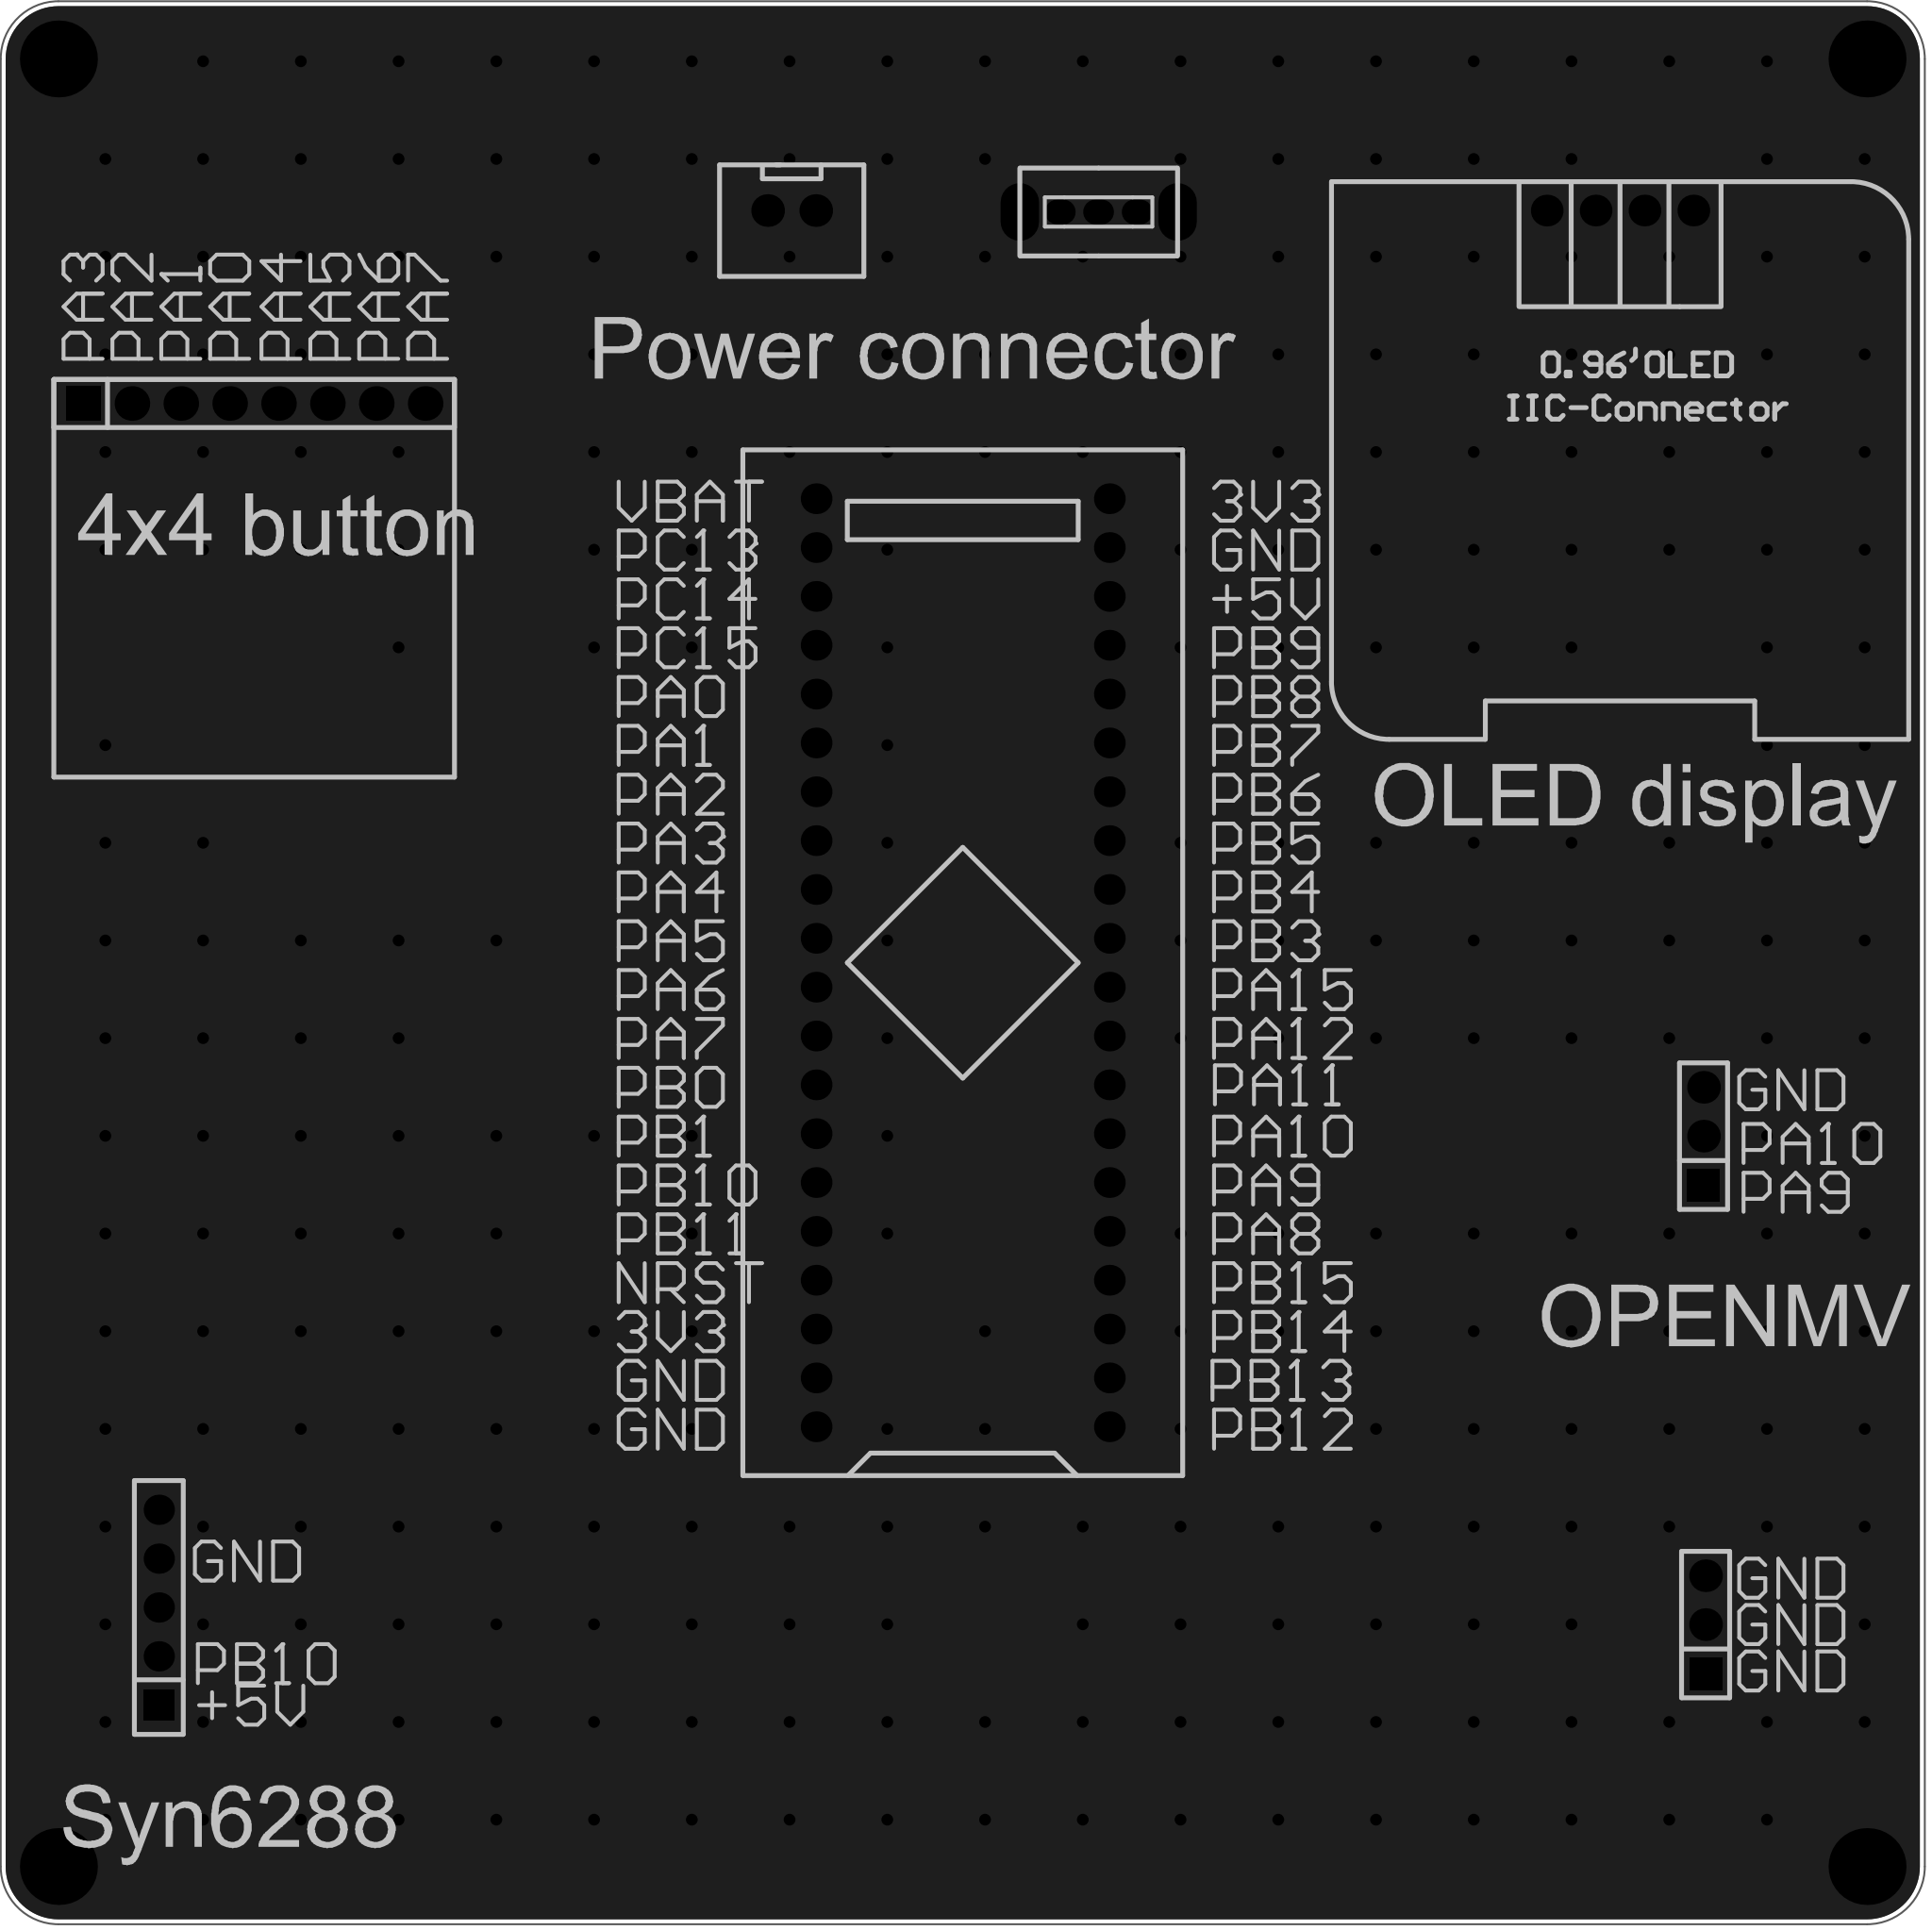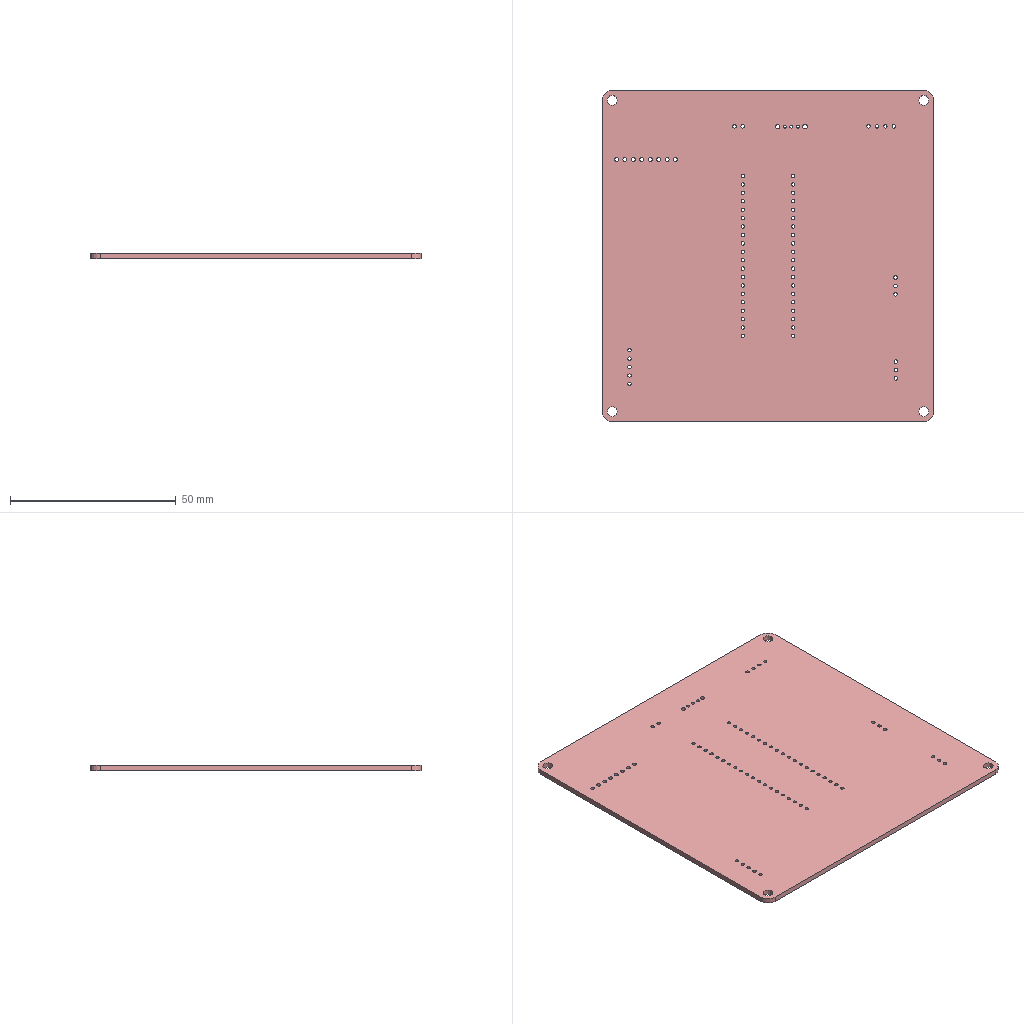Circuit board layout | Altium Designer | box 100 x 100 x 1.6 mm
Layer stack:
# Altium Designer layer stack of  (unit mm; dielectric type: 0 none, 1 core, 2 prepreg, 3 surface material)
index,name,kind,layer,copper_thickness_mm,dielectric_type,dielectric_thickness_mm,dielectric_material,dielectric_constant
0,Top Paste Mask Layer,other,,,,,,
1,Top Silkscreen Layer,other,,,,,,
2,Top Solder Mask Layer,dielectric,,,3,0.01,,3.3
3,Top Layer,copper,Top Layer,0.035,,,,
4,Dielectric1,dielectric,,,3,1.51,FR4,4.5
5,Bottom Layer,copper,Bottom Layer,0.035,,,,
6,Bottom Solder Mask Layer,dielectric,,,3,0.01,,3.3
7,Bottom Silkscreen Layer,other,,,,,,
8,Bottom Paste Mask Layer,other,,,,,,
# drill layer pairs: low layer,high layer
drill_pair,Top Layer,Bottom Layer
Part placement:
Designator,Comment,Layer,Footprint,Center-X(mm),Center-Y(mm),Rotation
U1,STM32F103C8T6-Card,TopLayer,CONN-TH_L53.3-W22.9_STM32F103C8T6-CARD,141.351,130.937,90
OLED1,,TopLayer,0.96OLED_4P,175.514,170.053,0
CN4,XH2.54*2P_Through-hole,TopLayer,CONN-TH_2P-P2.50-XH2.54-2P,132.461,170.053,0
SW5,,TopLayer,拨动开关,148.417,169.978,0
插槽出版子,,TopLayer,HDR-TH_5P-P2.54-V-F,99.568,97.409,90
H5,,TopLayer,HDR-TH_3P-P2.54-V-M,179.852,121.92,90
H6,,TopLayer,HDR-TH_8P-P2.54-V-F-1,104.521,160.02,0
H1,,TopLayer,HDR-TH_3P-P2.54-V-M,179.959,96.52,90
Pad and via stacks:
# Altium Designer via and pad stacks of  (unit mm). Each distinct definition once, with the count of objects using it.
# via: kind,start_layer,end_layer,hole_mm,diameter_mm,mode(0 simple;1 top-mid-bottom;2 full stack),diameter_per_layer,count,example_net
# pad: kind,layer,hole_mm,hole_type(0 round;1 square;2 slot),plating,top_size,top_shape(1 round;2 rect;3 octagon;9 rounded rect),mid_size,bottom_size,mode,footprint,size_per_layer,count,example
pad,Multi-Layer,3,0,plated,4x4,1,4x4,4x4,0,,,4,1
pad,Multi-Layer,1,0,plated,1.6x1.6,1,1.6x1.6,1.6x1.6,0,CONN-TH_L53.3-W22.9_STM32F103C8T6-CARD,,40,U1.1
pad,Multi-Layer,1,0,plated,1.65x1.65,1,1.65x1.65,1.65x1.65,0,0.96OLED_4P,,4,OLED1.4
pad,Multi-Layer,1.05,0,plated,1.7x1.7,1,1.7x1.7,1.7x1.7,0,CONN-TH_2P-P2.50-XH2.54-2P,,2,CN4.2
pad,Multi-Layer,0.8992,0,plated,1.6x1.3,1,1.6x1.3,1.6x1.3,0,\u00B2\u00A6\u00B6\u00AF\u00BF\u00AA\u00B9\u00D8,,3,SW5.1
pad,Multi-Layer,1.3,0,plated,3x1.999,1,3x1.999,3x1.999,0,\u00B2\u00A6\u00B6\u00AF\u00BF\u00AA\u00B9\u00D8,,2,SW5.4
pad,Multi-Layer,1.02,0,plated,1.575x1.575,1,1.575x1.575,1.575x1.575,0,HDR-TH_5P-P2.54-V-F,,4,\u63D2\u69FD\u51FA\u7248\u5B50.5
pad,Multi-Layer,1.02,0,plated,1.575x1.575,2,1.575x1.575,1.575x1.575,0,HDR-TH_5P-P2.54-V-F,,1,\u63D2\u69FD\u51FA\u7248\u5B50.1
pad,Multi-Layer,1.1,0,plated,1.7x1.7,2,1.7x1.7,1.7x1.7,0,HDR-TH_3P-P2.54-V-M,,2,H5.1
pad,Multi-Layer,1.1,0,plated,1.7x1.7,1,1.7x1.7,1.7x1.7,0,HDR-TH_3P-P2.54-V-M,,4,H5.2
pad,Multi-Layer,1.2,0,plated,1.8x1.8,2,1.8x1.8,1.8x1.8,0,HDR-TH_8P-P2.54-V-F-1,,1,H6.1
pad,Multi-Layer,1.2,0,plated,1.8x1.8,1,1.8x1.8,1.8x1.8,0,HDR-TH_8P-P2.54-V-F-1,,7,H6.2
via,Top Layer,Bottom Layer,0.3048,0.61,0,,286,GND
Copper pours:
name,layer,net,type(0 solid;1 hatched;2 none)
Bottom Layer-GND,Bottom Layer,GND,0
Top Layer-GND,Top Layer,GND,0
Design rules, without the lines most boards share:
# Altium Designer design rules of  (exported by Altium Designer, unit mm)
# columns: name | kind | enabled | priority | scope1 | scope2 | descriptor | typed fields (field=value)
Copper_copperRegion_copperThickness1oz | 0 | disabled | 4 | All | All | Clearance Constraint (Gap=5.984mil) (Disabled)(All),(All) | gap=0.152
Copper_copperRegion_copperThickness1oz_1 | 63 | disabled | 4 | All | All | Board Clearance Constraint (Gap=0mil) (Disabled)(All) |
Copper_copperRegion_Copper_copperRegion | 0 | disabled | 5 | All | All | Clearance Constraint (Gap=5.984mil) (Disabled)(All),(All) | gap=0.152
Copper_copperRegion_Copper_copperRegion_1 | 63 | disabled | 5 | All | All | Board Clearance Constraint (Gap=0mil) (Disabled)(All) |
copperThickness1oz | 0 | enabled | 6 | All | All | Clearance Constraint (Gap=5.984mil) (All),(All) | gap=0.152
copperThickness1oz_1 | 63 | enabled | 6 | All | All | Board Clearance Constraint (Gap=0mil) (All) |
copperRegion_copperThickness1oz | 20 | disabled | 1 | All | All | Polygon Connect Rule(Relief Connect )(Conductor Width=10mil) (Relief Angle=90 Angle) (Entries=4) (Air Gap Width=10mil) (Disabled)(All),(All) | connect_style(0=relief,1=direct,2=none)=0 relief_conductor_width=0.254 relief_entries=4
copperRegion_Copper_copperRegion | 20 | disabled | 2 | All | All | Polygon Connect Rule(Relief Connect )(Conductor Width=10mil) (Relief Angle=90 Angle) (Entries=4) (Air Gap Width=10mil) (Disabled)(All),(All) | connect_style(0=relief,1=direct,2=none)=0 relief_conductor_width=0.254 relief_entries=4
copperRegion | 20 | enabled | 3 | All | All | Polygon Connect Rule(Relief Connect )(Conductor Width=10mil) (Relief Angle=90 Angle) (Entries=4) (Air Gap Width=10mil) (All),(All) | connect_style(0=relief,1=direct,2=none)=0 relief_conductor_width=0.254 relief_entries=4